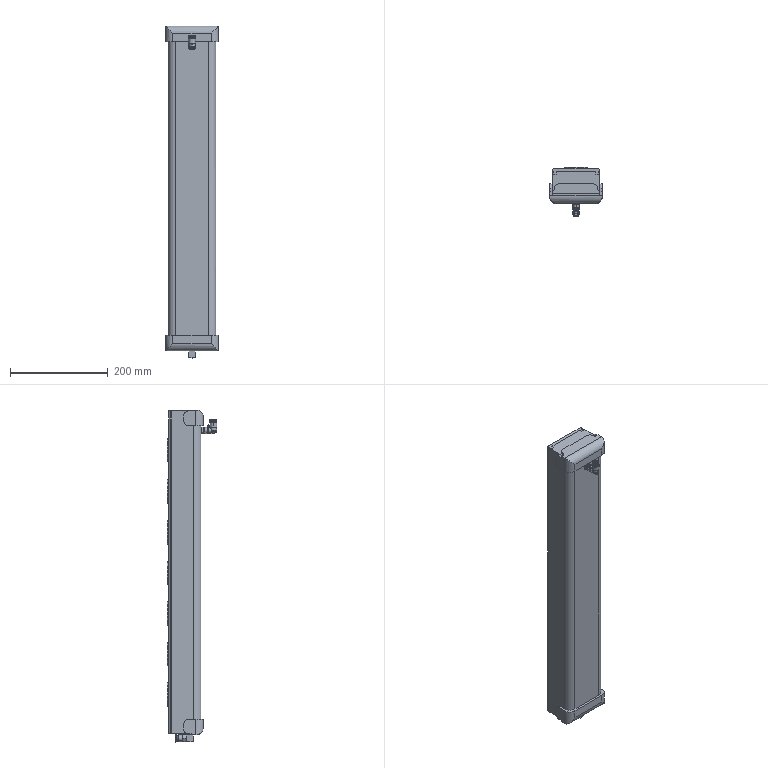Part | SolidWorks | 24 solids | 1418 faces | box 107.82 x 101.739 x 678.552 mm | volume 1521216 mm3 | plane 783 | cylinder 432 | cone 126 | torus 40 | spline 27 | sphere 10 | commonest cylinder face diameters 10.222 x56 30.787 x56 8.17 x28 6.779 x24 30 x20 7.866 x19